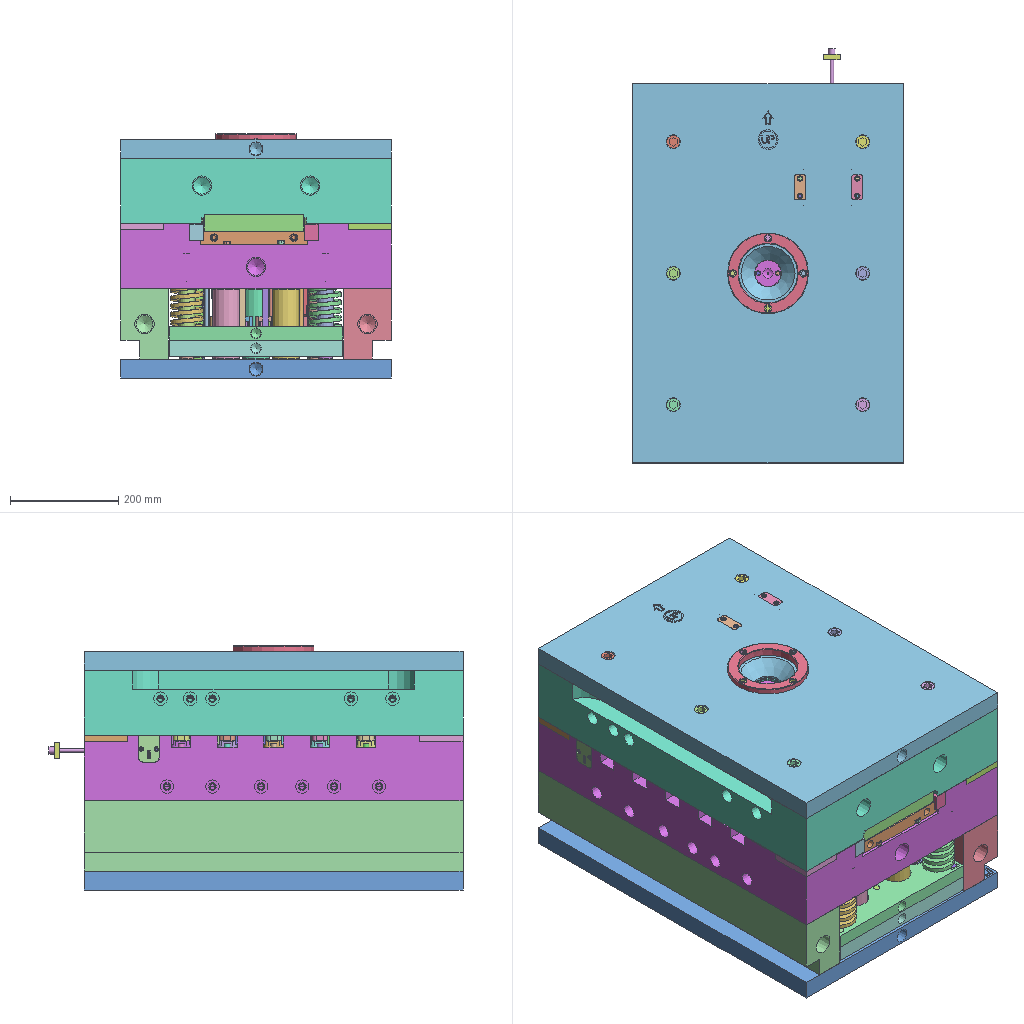Assembly | STEP file | 211 different items | 548 placed | box 500 x 765 x 451 mm
Parts list (item | name | quantity | parent item | size | volume):
1 | AA | x1 | in 11HPX006-GM-LH-2012.04.18_objects | 500 x 700 x 120 mm | 27100878 mm3
2 | AD | x1 | in 11HPX006-GM-LH-2012.04.18_objects | 500 x 700 x 35 mm | 11840083 mm3
3 | BD | x1 | in 11HPX006-GM-LH-2012.04.18_objects | 500 x 700 x 35 mm | 11472852 mm3
4 | CC01 | x1 | in 11HPX006-GM-LH-2012.04.18_objects | 88 x 700 x 130 mm | 6902512 mm3
5 | CC02 | x1 | in 11HPX006-GM-LH-2012.04.18_objects | 88 x 700 x 130 mm | 6902512 mm3
6 | DDZ10 | x1 | in 11HPX006-GM-LH-2012.04.18_objects | 208 x 339 x 231.203 mm | 51713 mm3
7 | DDZ8 | x1 | in 11HPX006-GM-LH-2012.04.18_objects | 132.5 x 223 x 215.546 mm | 32090 mm3
8 | DZDB | x1 | in 11HPX006-GM-LH-2012.04.18_objects | 320 x 700 x 30 mm | 5578536 mm3
9 | DZMB | x1 | in 11HPX006-GM-LH-2012.04.18_objects | 320 x 700 x 25 mm | 4227147 mm3
10 | FTH60.00-145.00 | x4 | in 11HPX006-GM-LH-2012.04.18_objects | 60 x 60.001 x 130 mm | 125930 mm3
11 | KBQ13.00 | x4 | in 11HPX006-GM-LH-2012.04.18_objects | 13 x 13 x 39.94 mm | 3312 mm3
12 | LJD | x10 | in 11HPX006-GM-LH-2012.04.18_objects | 25 x 25 x 15.25 mm | 2621 mm3
13 | M10.00-25.00 | x4 | in 11HPX006-GM-LH-2012.04.18_objects | 16 x 16 x 34 mm | 3561 mm3
14 | M10.00-35.00 | x12 | in 11HPX006-GM-LH-2012.04.18_objects | 16 x 16 x 44 mm | 4346 mm3
15 | M16.00-80.00 | x9 | in 11HPX006-GM-LH-2012.04.18_objects | 24 x 24 x 80.203 mm | 18728 mm3
16 | M16.00-95.00 | x11 | in 11HPX006-GM-LH-2012.04.18_objects | 24 x 24 x 93.469 mm | 21396 mm3
17 | M4.00-25.00 | x2 | in 11HPX006-GM-LH-2012.04.18_objects | 29 x 7 x 7 mm | 447.208 mm3
18 | M5.00-20 | x2 | in 11HPX006-GM-LH-2012.04.18_objects | 128.111 x 253.437 x 184.519 mm | 1683 mm3
19 | M5.00-30.00 | x4 | in 11HPX006-GM-LH-2012.04.18_objects | 8.5 x 8.5 x 29 mm | 713.513 mm3
20 | M6.00-30.00 | x2 | in 11HPX006-GM-LH-2012.04.18_objects | 10 x 10 x 26 mm | 965.752 mm3
21 | M6.00-50.00 | x1 | in 11HPX006-GM-LH-2012.04.18_objects | 10 x 10 x 49.34 mm | 1626 mm3
22 | M6.00-80.00 | x1 | in 11HPX006-GM-LH-2012.04.18_objects | 10 x 10 x 76 mm | 2379 mm3
23 | M8.00-35.00 | x38 | in 11HPX006-GM-LH-2012.04.18_objects | 13 x 13 x 35 mm | 2247 mm3
24 | M8.00-45.00 | x19 | in 11HPX006-GM-LH-2012.04.18_objects | 13 x 13 x 45 mm | 2750 mm3
25 | M8.00-75.00 | x8 | in 11HPX006-GM-LH-2012.04.18_objects | 13 x 13 x 75 mm | 4258 mm3
26 | MPPJ | x4 | in 11HPX006-GM-LH-2012.04.18_objects | 167 x 115 x 439 mm | 666925 mm3
27 | WTM10.00 | x2 | in 11HPX006-GM-LH-2012.04.18_objects | 10 x 10 x 10 mm | 660.357 mm3
28 | solid 1 | x2 | in 11HPX006-GM-LH-2012.04.18_objects | 25 x 42.455 x 97.821 mm | 32760 mm3
29 | solid 10 | x4 | in 11HPX006-GM-LH-2012.04.18_objects | 60 x 55.425 x 22 mm | 49802 mm3
30 | solid 100 | x1 | in 11HPX006-GM-LH-2012.04.18_objects | 64 x 36 x 20 mm | 38384 mm3
31 | solid 101 | x1 | in 11HPX006-GM-LH-2012.04.18_objects | 36 x 64 x 20 mm | 38384 mm3
32 | solid 102 | x1 | in 11HPX006-GM-LH-2012.04.18_objects | 64 x 36 x 20 mm | 37344 mm3
33 | solid 103 | x1 | in 11HPX006-GM-LH-2012.04.18_objects | 64 x 36 x 20 mm | 38230 mm3
34 | solid 104 | x1 | in 11HPX006-GM-LH-2012.04.18_objects | 64 x 36 x 20 mm | 38230 mm3
35 | solid 105 | x1 | in 11HPX006-GM-LH-2012.04.18_objects | 64 x 36 x 20 mm | 38008 mm3
36 | solid 106 | x1 | in 11HPX006-GM-LH-2012.04.18_objects | 64 x 36 x 20 mm | 37201 mm3
37 | solid 107 | x1 | in 11HPX006-GM-LH-2012.04.18_objects | 25 x 65 x 15 mm | 20230 mm3
38 | solid 108 | x20 | in 11HPX006-GM-LH-2012.04.18_objects | 12 x 5 x 12 mm | 621.825 mm3
39 | solid 109 | x10 | in 11HPX006-GM-LH-2012.04.18_objects | 5 x 20 x 5 mm | 392.699 mm3
40 | solid 11 | x1 | in 11HPX006-GM-LH-2012.04.18_objects | 70 x 31 x 60 mm | 72181 mm3
41 | solid 110 | x2 | in 11HPX006-GM-LH-2012.04.18_objects | 26.632 x 16 x 191.753 mm | 29798 mm3
42 | solid 111 | x1 | in 11HPX006-GM-LH-2012.04.18_objects | 25 x 40 x 43 mm | 32572 mm3
43 | solid 112 | x1 | in 11HPX006-GM-LH-2012.04.18_objects | 26.632 x 16 x 191.753 mm | 29798 mm3
44 | solid 113 | x1 | in 11HPX006-GM-LH-2012.04.18_objects | 25 x 40 x 43 mm | 32572 mm3
45 | solid 114 | x1 | in 11HPX006-GM-LH-2012.04.18_objects | 26.632 x 16 x 191.753 mm | 29798 mm3
46 | solid 115 | x1 | in 11HPX006-GM-LH-2012.04.18_objects | 25 x 40 x 43 mm | 32572 mm3
47 | solid 116 | x1 | in 11HPX006-GM-LH-2012.04.18_objects | 26.632 x 16 x 191.753 mm | 29797 mm3
48 | solid 117 | x1 | in 11HPX006-GM-LH-2012.04.18_objects | 25 x 40 x 43 mm | 32572 mm3
49 | solid 118 | x1 | in 11HPX006-GM-LH-2012.04.18_objects | 25 x 40 x 43 mm | 32572 mm3
50 | solid 119 | x1 | in 11HPX006-GM-LH-2012.04.18_objects | 25 x 40 x 43 mm | 32572 mm3
51 | solid 12 | x1 | in 11HPX006-GM-LH-2012.04.18_objects | 70 x 31 x 60 mm | 72181 mm3
52 | solid 120 | x1 | in 11HPX006-GM-LH-2012.04.18_objects | 25.771 x 16 x 182.341 mm | 28258 mm3
53 | solid 121 | x1 | in 11HPX006-GM-LH-2012.04.18_objects | 25 x 40 x 43 mm | 32572 mm3
54 | solid 122 | x1 | in 11HPX006-GM-LH-2012.04.18_objects | 25.771 x 16 x 182.341 mm | 28258 mm3
55 | solid 123 | x1 | in 11HPX006-GM-LH-2012.04.18_objects | 25 x 40 x 43 mm | 32572 mm3
56 | solid 124 | x7 | in 11HPX006-GM-LH-2012.04.18_objects | 20 x 4 x 4 mm | 251.327 mm3
57 | solid 125 | x14 | in 11HPX006-GM-LH-2012.04.18_objects | 5 x 12 x 12 mm | 657.168 mm3
58 | solid 126 | x1 | in 11HPX006-GM-LH-2012.04.18_objects | 36 x 25 x 43 mm | 28272 mm3
59 | solid 127 | x1 | in 11HPX006-GM-LH-2012.04.18_objects | 10 x 17.865 x 190.084 mm | 15194 mm3
60 | solid 128 | x1 | in 11HPX006-GM-LH-2012.04.18_objects | 36 x 25 x 43 mm | 28272 mm3
61 | solid 129 | x1 | in 11HPX006-GM-LH-2012.04.18_objects | 36 x 25 x 43 mm | 28272 mm3
62 | solid 13 | x1 | in 11HPX006-GM-LH-2012.04.18_objects | 20 x 76.984 x 20 mm | 26313 mm3
63 | solid 130 | x1 | in 11HPX006-GM-LH-2012.04.18_objects | 55 x 30 x 43 mm | 51024 mm3
64 | solid 131 | x4 | in 11HPX006-GM-LH-2012.04.18_objects | 3 x 12 x 12 mm | 394.301 mm3
65 | solid 132 | x2 | in 11HPX006-GM-LH-2012.04.18_objects | 16 x 4 x 4 mm | 201.062 mm3
66 | solid 133 | x1 | in 11HPX006-GM-LH-2012.04.18_objects | 36 x 25 x 43 mm | 28272 mm3
67 | solid 134 | x1 | in 11HPX006-GM-LH-2012.04.18_objects | 36 x 25 x 43 mm | 28272 mm3
68 | solid 135 | x1 | in 11HPX006-GM-LH-2012.04.18_objects | 36 x 25 x 43 mm | 28272 mm3
69 | solid 136 | x1 | in 11HPX006-GM-LH-2012.04.18_objects | 36 x 25 x 43 mm | 28272 mm3
70 | solid 137 | x1 | in 11HPX006-GM-LH-2012.04.18_objects | 25.825 x 16 x 182.529 mm | 28690 mm3
71 | solid 138 | x1 | in 11HPX006-GM-LH-2012.04.18_objects | 14 x 19.289 x 179.041 mm | 24279 mm3
72 | solid 139 | x2 | in 11HPX006-GM-LH-2012.04.18_objects | 21 x 47 x 10 mm | 8523 mm3
73 | solid 14 | x1 | in 11HPX006-GM-LH-2012.04.18_objects | 17 x 65 x 20 mm | 17619 mm3
74 | solid 141 | x1 | in 11HPX006-GM-LH-2012.04.18_objects | 73.616 x 36 x 30 mm | 41988 mm3
75 | solid 142 | x1 | in 11HPX006-GM-LH-2012.04.18_objects | 73.616 x 36 x 30 mm | 41988 mm3
76 | solid 143 | x1 | in 11HPX006-GM-LH-2012.04.18_objects | 73.616 x 36 x 30 mm | 41988 mm3
77 | solid 144 | x1 | in 11HPX006-GM-LH-2012.04.18_objects | 140 x 75 x 59 mm | 401868 mm3
78 | solid 145 | x1 | in 11HPX006-GM-LH-2012.04.18_objects | 177 x 14.981 x 25 mm | 35338 mm3
79 | solid 15 | x1 | in 11HPX006-GM-LH-2012.04.18_objects | 155 x 126.362 x 50 mm | 501554 mm3
80 | solid 152 | x1 | in 11HPX006-GM-LH-2012.04.18_objects | 39 x 60 x 43 mm | 71381 mm3
81 | solid 153 | x14 | in 11HPX006-GM-LH-2012.04.18_objects | 12 x 12 x 17.55 mm | 614.689 mm3
82 | solid 154 | x23 | in 11HPX006-GM-LH-2012.04.18_objects | 12 x 12 x 15.55 mm | 558.14 mm3
83 | solid 155 | x6 | in 11HPX006-GM-LH-2012.04.18_objects | 16 x 16 x 66.6 mm | 6156 mm3
84 | solid 156 | x2 | in 11HPX006-GM-LH-2012.04.18_objects | 16 x 16 x 64.4 mm | 5983 mm3
85 | solid 157 | x2 | in 11HPX006-GM-LH-2012.04.18_objects | 16 x 16 x 40.4 mm | 4098 mm3
86 | solid 158 | x5 | in 11HPX006-GM-LH-2012.04.18_objects | 16 x 16 x 68 mm | 6266 mm3
87 | solid 159 | x1 | in 11HPX006-GM-LH-2012.04.18_objects | 16 x 16 x 68 mm | 6098 mm3
88 | solid 16 | x1 | in 11HPX006-GM-LH-2012.04.18_objects | 139 x 12.642 x 24 mm | 19581 mm3
89 | solid 160 | x3 | in 11HPX006-GM-LH-2012.04.18_objects | 12 x 17.22 x 12.589 mm | 558.14 mm3
90 | solid 161 | x4 | in 11HPX006-GM-LH-2012.04.18_objects | 13 x 13 x 45 mm | 2785 mm3
91 | solid 162 | x12 | in 11HPX006-GM-LH-2012.04.18_objects | 13 x 13 x 40 mm | 2534 mm3
92 | solid 163 | x16 | in 11HPX006-GM-LH-2012.04.18_objects | 13 x 13 x 31 mm | 2081 mm3
93 | solid 164 | x4 | in 11HPX006-GM-LH-2012.04.18_objects | 13 x 13 x 35 mm | 2282 mm3
94 | solid 165 | x4 | in 11HPX006-GM-LH-2012.04.18_objects | 16 x 16 x 48 mm | 4695 mm3
95 | solid 166 | x2 | in 11HPX006-GM-LH-2012.04.18_objects | 16 x 16 x 73 mm | 6658 mm3
96 | solid 167 | x2 | in 11HPX006-GM-LH-2012.04.18_objects | 16 x 16 x 77 mm | 6973 mm3
97 | solid 17 | x1 | in 11HPX006-GM-LH-2012.04.18_objects | 197 x 126.362 x 50 mm | 664988 mm3
98 | solid 175 | x4 | in 11HPX006-GM-LH-2012.04.18_objects | 40 x 40 x 130 mm | 162047 mm3
99 | solid 177 | x8 | in 11HPX006-GM-LH-2012.04.18_objects | 50 x 50 x 130 mm | 253962 mm3
100 | solid 178 | x4 | in 11HPX006-GM-LH-2012.04.18_objects | 30 x 30 x 20 mm | 10459 mm3
101 | solid 18 | x1 | in 11HPX006-GM-LH-2012.04.18_objects | 184 x 65 x 55 mm | 526326 mm3
102 | solid 183 | x1 | in 11HPX006-GM-LH-2012.04.18_objects | 25 x 38 x 49.5 mm | 43620 mm3
103 | solid 184 | x4 | in 11HPX006-GM-LH-2012.04.18_objects | 20 x 20 x 15 mm | 4712 mm3
104 | solid 185 | x1 | in 11HPX006-GM-LH-2012.04.18_objects | 7.25 x 93.183 x 8.999 mm | 1776 mm3
105 | solid 186 | x1 | in 11HPX006-GM-LH-2012.04.18_objects | 500 x 700 x 120 mm | 24510604 mm3
106 | solid 187 | x9 | in 11HPX006-GM-LH-2012.04.18_objects | 11 x 11 x 22 mm | 1002 mm3
107 | solid 188 | x4 | in 11HPX006-GM-LH-2012.04.18_objects | 20 x 20 x 20 mm | 5479 mm3
108 | solid 19 | x1 | in 11HPX006-GM-LH-2012.04.18_objects | 25 x 90 x 30 mm | 60451 mm3
109 | solid 191 | x1 | in 11HPX006-GM-LH-2012.04.18_objects | 34 x 79.555 x 65 mm | 95277 mm3
110 | solid 192 | x4 | in 11HPX006-GM-LH-2012.04.18_objects | 3 x 8.885 x 6 mm | 138.722 mm3
111 | solid 193 | x2 | in 11HPX006-GM-LH-2012.04.18_objects | 13.5 x 3 x 3 mm | 95.426 mm3
112 | solid 194 | x1 | in 11HPX006-GM-LH-2012.04.18_objects | 25 x 21.5 x 19.435 mm | 7259 mm3
113 | solid 195 | x1 | in 11HPX006-GM-LH-2012.04.18_objects | 25 x 21.5 x 19.435 mm | 7243 mm3
114 | solid 196 | x1 | in 11HPX006-GM-LH-2012.04.18_objects | 25 x 21.5 x 21.524 mm | 7409 mm3
115 | solid 197 | x1 | in 11HPX006-GM-LH-2012.04.18_objects | 25 x 21.5 x 21.524 mm | 7409 mm3
116 | solid 198 | x1 | in 11HPX006-GM-LH-2012.04.18_objects | 25 x 21.5 x 21.524 mm | 7423 mm3
117 | solid 199 | x1 | in 11HPX006-GM-LH-2012.04.18_objects | 25 x 21.516 x 19.435 mm | 7268 mm3
118 | solid 2 | x1 | in 11HPX006-GM-LH-2012.04.18_objects | 10 x 10 x 73.694 mm | 2193 mm3
119 | solid 20 | x1 | in 11HPX006-GM-LH-2012.04.18_objects | 25 x 90 x 30 mm | 54142 mm3
120 | solid 200 | x1 | in 11HPX006-GM-LH-2012.04.18_objects | 25 x 21.516 x 19.435 mm | 7252 mm3
121 | solid 201 | x1 | in 11HPX006-GM-LH-2012.04.18_objects | 25 x 21.5 x 21.524 mm | 7423 mm3
122 | solid 202 | x2 | in 11HPX006-GM-LH-2012.04.18_objects | 3.318 x 2.972 x 4.241 mm | 13.916 mm3
123 | solid 203 | x1 | in 11HPX006-GM-LH-2012.04.18_objects | 60 x 30 x 60 mm | 64241 mm3
124 | solid 204 | x1 | in 11HPX006-GM-LH-2012.04.18_objects | 60 x 30 x 60 mm | 64241 mm3
125 | solid 205 | x1 | in 11HPX006-GM-LH-2012.04.18_objects | 300 x 520 x 85 mm | 8735369 mm3
126 | solid 207 | x1 | in 11HPX006-GM-LH-2012.04.18_objects | 300 x 520 x 75.001 mm | 8769898 mm3
127 | solid 208 | x1 | in 11HPX006-GM-LH-2012.04.18_objects | 8 x 50 x 8 mm | 2513 mm3
128 | solid 209 | x1 | in 11HPX006-GM-LH-2012.04.18_objects | 31 x 10 x 31 mm | 9107 mm3
129 | solid 21 | x1 | in 11HPX006-GM-LH-2012.04.18_objects | 25 x 90 x 30.004 mm | 49415 mm3
130 | solid 210 | x1 | in 11HPX006-GM-LH-2012.04.18_objects | 13 x 147.06 x 13 mm | 6410 mm3
131 | solid 211 | x1 | in 11HPX006-GM-LH-2012.04.18_objects | 26.578 x 10.027 x 14.799 mm | 1219 mm3
132 | solid 212 | x1 | in 11HPX006-GM-LH-2012.04.18_objects | 3.206 x 2.939 x 4.252 mm | 13.592 mm3
133 | solid 213 | x1 | in 11HPX006-GM-LH-2012.04.18_objects | 3.206 x 2.939 x 4.314 mm | 13.64 mm3
134 | solid 214 | x1 | in 11HPX006-GM-LH-2012.04.18_objects | 114.278 x 185.224 x 7.51 mm | 11384 mm3
135 | solid 215 | x1 | in 11HPX006-GM-LH-2012.04.18_objects | 26.632 x 10.173 x 15.494 mm | 1276 mm3
136 | solid 216 | x1 | in 11HPX006-GM-LH-2012.04.18_objects | 12.653 x 1.816 x 0.4476 mm | 2.762 mm3
137 | solid 217 | x2 | in 11HPX006-GM-LH-2012.04.18_objects | 7.264 x 1.563 x 4.422 mm | 23.265 mm3
138 | solid 218 | x2 | in 11HPX006-GM-LH-2012.04.18_objects | 31.5 x 4.648 x 7.129 mm | 682.585 mm3
139 | solid 219 | x1 | in 11HPX006-GM-LH-2012.04.18_objects | - | 1019 mm3
140 | solid 22 | x1 | in 11HPX006-GM-LH-2012.04.18_objects | 25 x 90 x 30.004 mm | 57330 mm3
141 | solid 220 | x1 | in 11HPX006-GM-LH-2012.04.18_objects | - | 199.733 mm3
142 | solid 221 | x1 | in 11HPX006-GM-LH-2012.04.18_objects | 26.698 x 10.392 x 16.548 mm | 1362 mm3
143 | solid 222 | x1 | in 11HPX006-GM-LH-2012.04.18_objects | 32.172 x 3.969 x 3.297 mm | 218.611 mm3
144 | solid 223 | x1 | in 11HPX006-GM-LH-2012.04.18_objects | 117.1 x 176.873 x 3.297 mm | 10209 mm3
145 | solid 224 | x1 | in 11HPX006-GM-LH-2012.04.18_objects | 87.441 x 176.873 x 5.302 mm | 4897 mm3
146 | solid 23 | x1 | in 11HPX006-GM-LH-2012.04.18_objects | 25.771 x 16 x 182.341 mm | 28258 mm3
147 | solid 24 | x1 | in 11HPX006-GM-LH-2012.04.18_objects | 25.771 x 16 x 182.341 mm | 28258 mm3
148 | solid 25 | x1 | in 11HPX006-GM-LH-2012.04.18_objects | 10 x 17.713 x 187.185 mm | 14965 mm3
149 | solid 26 | x1 | in 11HPX006-GM-LH-2012.04.18_objects | 10 x 17.589 x 184.804 mm | 14786 mm3
150 | solid 27 | x1 | in 11HPX006-GM-LH-2012.04.18_objects | 10 x 17.491 x 182.939 mm | 14658 mm3
151 | solid 28 | x1 | in 11HPX006-GM-LH-2012.04.18_objects | 10 x 17.865 x 190.084 mm | 15194 mm3
152 | solid 29 | x1 | in 11HPX006-GM-LH-2012.04.18_objects | 10 x 17.713 x 187.185 mm | 14964 mm3
153 | solid 3 | x6 | in 11HPX006-GM-LH-2012.04.18_objects | 55 x 20 x 25 mm | 22425 mm3
154 | solid 30 | x1 | in 11HPX006-GM-LH-2012.04.18_objects | 10 x 17.589 x 184.804 mm | 14786 mm3
155 | solid 31 | x1 | in 11HPX006-GM-LH-2012.04.18_objects | 10 x 17.491 x 182.939 mm | 14658 mm3
156 | solid 32 | x1 | in 11HPX006-GM-LH-2012.04.18_objects | 170 x 100 x 15 mm | 197483 mm3
157 | solid 33 | x4 | in 11HPX006-GM-LH-2012.04.18_objects | 10 x 10 x 28 mm | 1005 mm3
158 | solid 34 | x2 | in 11HPX006-GM-LH-2012.04.18_objects | 25 x 25 x 119 mm | 38365 mm3
159 | solid 35 | x2 | in 11HPX006-GM-LH-2012.04.18_objects | 25 x 25 x 106 mm | 34281 mm3
160 | solid 36 | x2 | in 11HPX006-GM-LH-2012.04.18_objects | 17 x 17 x 99.469 mm | 11303 mm3
161 | solid 37 | x2 | in 11HPX006-GM-LH-2012.04.18_objects | 23 x 23 x 28 mm | 4924 mm3
162 | solid 38 | x1 | in 11HPX006-GM-LH-2012.04.18_objects | 27.996 x 50 x 19 mm | 19083 mm3
163 | solid 39 | x2 | in 11HPX006-GM-LH-2012.04.18_objects | 10 x 10 x 16.5 mm | 680.158 mm3
164 | solid 4 | x9 | in 11HPX006-GM-LH-2012.04.18_objects | 27.19 x 17 x 60.243 mm | 8744 mm3
165 | solid 40 | x1 | in 11HPX006-GM-LH-2012.04.18_objects | 170 x 100 x 15 mm | 236322 mm3
166 | solid 5 | x1 | in 11HPX006-GM-LH-2012.04.18_objects | 60 x 30 x 60 mm | 64241 mm3
167 | solid 55 | x4 | in 11HPX006-GM-LH-2012.04.18_objects | 30 x 30 x 180 mm | 84990 mm3
168 | solid 56 | x4 | in 11HPX006-GM-LH-2012.04.18_objects | 40 x 40 x 53 mm | 27190 mm3
169 | solid 58 | x5 | in 11HPX006-GM-LH-2012.04.18_objects | 55 x 36 x 6 mm | 10013 mm3
170 | solid 59 | x1 | in 11HPX006-GM-LH-2012.04.18_objects | 37 x 90.006 x 6 mm | 15565 mm3
171 | solid 6 | x1 | in 11HPX006-GM-LH-2012.04.18_objects | 70 x 31 x 60 mm | 72182 mm3
172 | solid 60 | x2 | in 11HPX006-GM-LH-2012.04.18_objects | 50 x 77 x 8 mm | 28929 mm3
173 | solid 61 | x2 | in 11HPX006-GM-LH-2012.04.18_objects | 80 x 77 x 8 mm | 47370 mm3
174 | solid 62 | x3 | in 11HPX006-GM-LH-2012.04.18_objects | 55 x 36 x 6 mm | 9848 mm3
175 | solid 64 | x1 | in 11HPX006-GM-LH-2012.04.18_objects | 100.766 x 36 x 30 mm | 52192 mm3
176 | solid 65 | x1 | in 11HPX006-GM-LH-2012.04.18_objects | 100.766 x 36 x 30 mm | 52192 mm3
177 | solid 66 | x1 | in 11HPX006-GM-LH-2012.04.18_objects | 100.766 x 36 x 30 mm | 52192 mm3
178 | solid 68 | x1 | in 11HPX006-GM-LH-2012.04.18_objects | 150 x 150 x 15 mm | 114637 mm3
179 | solid 69 | x4 | in 11HPX006-GM-LH-2012.04.18_objects | 13 x 13 x 29 mm | 1884 mm3
180 | solid 7 | x2 | in 11HPX006-GM-LH-2012.04.18_objects | 60 x 20 x 16 mm | 15370 mm3
181 | solid 70 | x1 | in 11HPX006-GM-LH-2012.04.18_objects | 50 x 50 x 126.59 mm | 43953 mm3
182 | solid 71 | x1 | in 11HPX006-GM-LH-2012.04.18_objects | 12.511 x 12.511 x 136.502 mm | 7240 mm3
183 | solid 73 | x1 | in 11HPX006-GM-LH-2012.04.18_objects | 25 x 100 x 50 mm | 71531 mm3
184 | solid 74 | x1 | in 11HPX006-GM-LH-2012.04.18_objects | 25 x 115 x 50 mm | 88592 mm3
185 | solid 75 | x1 | in 11HPX006-GM-LH-2012.04.18_objects | 25 x 105 x 50 mm | 77206 mm3
186 | solid 76 | x1 | in 11HPX006-GM-LH-2012.04.18_objects | 25 x 105 x 48.598 mm | 89861 mm3
187 | solid 77 | x1 | in 11HPX006-GM-LH-2012.04.18_objects | 25 x 105 x 48.598 mm | 89861 mm3
188 | solid 78 | x1 | in 11HPX006-GM-LH-2012.04.18_objects | 100 x 25 x 38.403 mm | 54742 mm3
189 | solid 79 | x1 | in 11HPX006-GM-LH-2012.04.18_objects | 100 x 25 x 38.403 mm | 51542 mm3
190 | solid 8 | x1 | in 11HPX006-GM-LH-2012.04.18_objects | 70 x 31 x 60 mm | 72181 mm3
191 | solid 80 | x1 | in 11HPX006-GM-LH-2012.04.18_objects | 25 x 105 x 48.598 mm | 89141 mm3
192 | solid 81 | x1 | in 11HPX006-GM-LH-2012.04.18_objects | 80 x 80 x 12 mm | 57233 mm3
193 | solid 82 | x3 | in 11HPX006-GM-LH-2012.04.18_objects | 80 x 80 x 12 mm | 57349 mm3
194 | solid 83 | x1 | in 11HPX006-GM-LH-2012.04.18_objects | 237.532 x 453.356 x 39.446 mm | 189015 mm3
195 | solid 84 | x1 | in 11HPX006-GM-LH-2012.04.18_objects | 7.5 x 20.479 x 119.36 mm | 7713 mm3
196 | solid 85 | x1 | in 11HPX006-GM-LH-2012.04.18_objects | 7.5 x 20.679 x 121.269 mm | 7846 mm3
197 | solid 86 | x2 | in 11HPX006-GM-LH-2012.04.18_objects | 25 x 40 x 43 mm | 32572 mm3
198 | solid 87 | x1 | in 11HPX006-GM-LH-2012.04.18_objects | 100.766 x 36 x 30 mm | 52192 mm3
199 | solid 88 | x1 | in 11HPX006-GM-LH-2012.04.18_objects | 100.766 x 36 x 30 mm | 52193 mm3
200 | solid 89 | x1 | in 11HPX006-GM-LH-2012.04.18_objects | 66 x 55 x 20 mm | 59537 mm3
201 | solid 9 | x1 | in 11HPX006-GM-LH-2012.04.18_objects | 70 x 31 x 60 mm | 72181 mm3
202 | solid 90 | x1 | in 11HPX006-GM-LH-2012.04.18_objects | 24 x 50 x 20 mm | 17760 mm3
203 | solid 91 | x1 | in 11HPX006-GM-LH-2012.04.18_objects | 24 x 50 x 20 mm | 17760 mm3
204 | solid 92 | x1 | in 11HPX006-GM-LH-2012.04.18_objects | 24 x 50 x 20 mm | 17760 mm3
205 | solid 93 | x1 | in 11HPX006-GM-LH-2012.04.18_objects | 24 x 50 x 20 mm | 17759 mm3
206 | solid 94 | x1 | in 11HPX006-GM-LH-2012.04.18_objects | 24 x 50 x 20 mm | 17759 mm3
207 | solid 95 | x1 | in 11HPX006-GM-LH-2012.04.18_objects | 24 x 50 x 20 mm | 17759 mm3
208 | solid 96 | x1 | in 11HPX006-GM-LH-2012.04.18_objects | 24 x 50 x 20 mm | 17760 mm3
209 | solid 97 | x1 | in 11HPX006-GM-LH-2012.04.18_objects | 64 x 36 x 20 mm | 38229 mm3
210 | solid 98 | x1 | in 11HPX006-GM-LH-2012.04.18_objects | 64 x 36 x 20 mm | 38229 mm3
211 | solid 99 | x1 | in 11HPX006-GM-LH-2012.04.18_objects | 64 x 36 x 20 mm | 38230 mm3